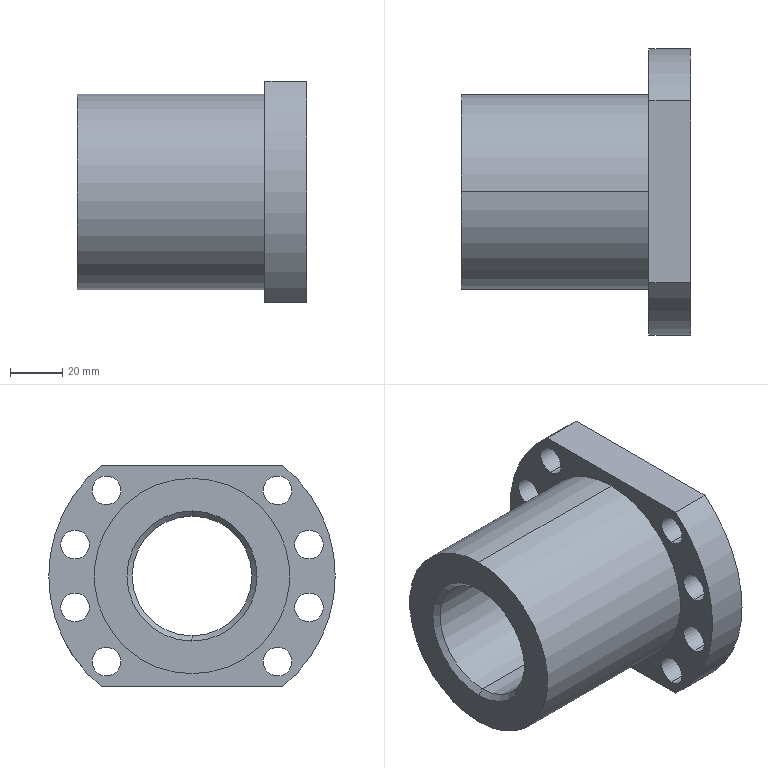Part | SolidWorks | features ICE 9, RefAxis 4, 3DProfileFeature 1, LockFeature 1, RevCut 1, Revolution 1 | 1 solid | 38 faces | box 88 x 110 x 85 mm | volume 291032 mm3 | cylinder 26 | cone 6 | plane 6 | commonest cylinder face diameters 11 x16 6 x2 6.647 x2 46 x2 75 x2 110 x2
STEP:
#1=CARTESIAN_POINT('',(80.,48.707,-24.284));
#2=VERTEX_POINT('',#1);
#3=CARTESIAN_POINT('',(80.,45.384,-30.04));
#4=VERTEX_POINT('',#3);
#5=CARTESIAN_POINT('',(80.,47.046,-27.162));
#6=DIRECTION('',(0.,-0.866,0.5));
#7=DIRECTION('',(0.,-0.5,-0.866));
#8=AXIS2_PLACEMENT_3D('',#5,#6,#7);
#9=CIRCLE('',#8,3.323);
#10=EDGE_CURVE('',#2,#4,#9,.T.);
#11=ORIENTED_EDGE('',*,*,#10,.F.);
#12=CARTESIAN_POINT('',(80.,35.437,-16.622));
#13=VERTEX_POINT('',#12);
#14=CARTESIAN_POINT('',(80.,49.293,-24.622));
#15=DIRECTION('',(0.,-0.866,0.5));
#16=VECTOR('',#15,1000.);
#17=LINE('',#14,#16);
#18=EDGE_CURVE('',#2,#13,#17,.T.);
#19=ORIENTED_EDGE('',*,*,#18,.T.);
#20=CARTESIAN_POINT('',(80.,32.113,-22.378));
#21=VERTEX_POINT('',#20);
#22=CARTESIAN_POINT('',(80.,33.775,-19.5));
#23=DIRECTION('',(0.,-0.866,0.5));
#24=DIRECTION('',(0.,-0.5,-0.866));
#25=AXIS2_PLACEMENT_3D('',#22,#23,#24);
#26=CIRCLE('',#25,3.323);
#27=EDGE_CURVE('',#13,#21,#26,.T.);
#28=ORIENTED_EDGE('',*,*,#27,.T.);
#29=CARTESIAN_POINT('',(80.,45.97,-30.378));
#30=DIRECTION('',(0.,-0.866,0.5));
#31=VECTOR('',#30,1000.);
#32=LINE('',#29,#31);
#33=EDGE_CURVE('',#4,#21,#32,.T.);
#34=ORIENTED_EDGE('',*,*,#33,.F.);
#35=EDGE_LOOP('',(#11,#19,#28,#34));
#36=FACE_OUTER_BOUND('',#35,.T.);
#37=CARTESIAN_POINT('',(80.,47.631,-27.5));
#38=DIRECTION('',(0.,-0.866,0.5));
#39=DIRECTION('',(0.,-0.5,-0.866));
#40=AXIS2_PLACEMENT_3D('',#37,#38,#39);
#41=CYLINDRICAL_SURFACE('',#40,3.323);
#42=ADVANCED_FACE('',(#36),#41,.F.);
#43=CARTESIAN_POINT('',(80.,35.275,-16.902));
#44=VERTEX_POINT('',#43);
#45=CARTESIAN_POINT('',(80.,32.275,-22.098));
#46=VERTEX_POINT('',#45);
#47=CARTESIAN_POINT('',(80.,33.775,-19.5));
#48=DIRECTION('',(0.,-0.866,0.5));
#49=DIRECTION('',(0.,-0.5,-0.866));
#50=AXIS2_PLACEMENT_3D('',#47,#48,#49);
#51=CIRCLE('',#50,3.);
#52=EDGE_CURVE('',#44,#46,#51,.T.);
#53=ORIENTED_EDGE('',*,*,#52,.F.);
#54=CARTESIAN_POINT('',(80.,21.248,-8.804));
#55=VERTEX_POINT('',#54);
#56=CARTESIAN_POINT('',(80.,49.131,-24.902));
#57=DIRECTION('',(0.,-0.866,0.5));
#58=VECTOR('',#57,1000.);
#59=LINE('',#56,#58);
#60=EDGE_CURVE('',#44,#55,#59,.T.);
#61=ORIENTED_EDGE('',*,*,#60,.T.);
#62=CARTESIAN_POINT('',(80.,18.248,-14.));
#63=VERTEX_POINT('',#62);
#64=CARTESIAN_POINT('',(80.,21.248,-8.804));
#65=CARTESIAN_POINT('',(79.804,21.248,-8.804));
#66=CARTESIAN_POINT('',(79.609,21.241,-8.821));
#67=CARTESIAN_POINT('',(79.222,21.211,-8.893));
#68=CARTESIAN_POINT('',(79.033,21.189,-8.947));
#69=CARTESIAN_POINT('',(78.672,21.13,-9.085));
#70=CARTESIAN_POINT('',(78.497,21.093,-9.171));
#71=CARTESIAN_POINT('',(78.169,21.004,-9.373));
#72=CARTESIAN_POINT('',(78.018,20.953,-9.487));
#73=CARTESIAN_POINT('',(77.742,20.837,-9.739));
#74=CARTESIAN_POINT('',(77.615,20.771,-9.879));
#75=CARTESIAN_POINT('',(77.397,20.629,-10.172));
#76=CARTESIAN_POINT('',(77.305,20.552,-10.327));
#77=CARTESIAN_POINT('',(77.154,20.386,-10.65));
#78=CARTESIAN_POINT('',(77.096,20.297,-10.819));
#79=CARTESIAN_POINT('',(77.02,20.114,-11.156));
#80=CARTESIAN_POINT('',(77.,20.019,-11.326));
#81=CARTESIAN_POINT('',(77.,19.82,-11.67));
#82=CARTESIAN_POINT('',(77.019,19.721,-11.838));
#83=CARTESIAN_POINT('',(77.095,19.52,-12.165));
#84=CARTESIAN_POINT('',(77.153,19.419,-12.327));
#85=CARTESIAN_POINT('',(77.303,19.221,-12.632));
#86=CARTESIAN_POINT('',(77.395,19.126,-12.776));
#87=CARTESIAN_POINT('',(77.613,18.942,-13.047));
#88=CARTESIAN_POINT('',(77.739,18.854,-13.174));
#89=CARTESIAN_POINT('',(78.015,18.694,-13.4));
#90=CARTESIAN_POINT('',(78.166,18.62,-13.501));
#91=CARTESIAN_POINT('',(78.494,18.49,-13.68));
#92=CARTESIAN_POINT('',(78.668,18.434,-13.755));
#93=CARTESIAN_POINT('',(79.029,18.343,-13.876));
#94=CARTESIAN_POINT('',(79.218,18.308,-13.922));
#95=CARTESIAN_POINT('',(79.605,18.26,-13.984));
#96=CARTESIAN_POINT('',(79.802,18.248,-14.));
#97=CARTESIAN_POINT('',(80.,18.248,-14.));
#98=B_SPLINE_CURVE_WITH_KNOTS('',3,(#64,#65,#66,#67,#68,#69,#70,#71,#72,#73,#74,#75,#76,#77,#78,#79,#80,#81,#82,#83,#84,#85,#86,#87,#88,#89,#90,#91,#92,#93,#94,#95,#96,#97),.UNSPECIFIED.,.F.,.F.,(4,2,2,2,2,2,2,2,2,2,2,2,2,2,2,2,4),(0.009389,0.009976,0.01056,0.01115,0.01174,0.01232,0.01291,0.0135,0.01408,0.01467,0.01526,0.01584,0.01643,0.01702,0.0176,0.01819,0.01878),.UNSPECIFIED.);
#99=EDGE_CURVE('',#55,#63,#98,.T.);
#100=ORIENTED_EDGE('',*,*,#99,.T.);
#101=CARTESIAN_POINT('',(80.,46.131,-30.098));
#102=DIRECTION('',(0.,-0.866,0.5));
#103=VECTOR('',#102,1000.);
#104=LINE('',#101,#103);
#105=EDGE_CURVE('',#46,#63,#104,.T.);
#106=ORIENTED_EDGE('',*,*,#105,.F.);
#107=EDGE_LOOP('',(#53,#61,#100,#106));
#108=FACE_OUTER_BOUND('',#107,.T.);
#109=CARTESIAN_POINT('',(80.,47.631,-27.5));
#110=DIRECTION('',(0.,-0.866,0.5));
#111=DIRECTION('',(0.,-0.5,-0.866));
#112=AXIS2_PLACEMENT_3D('',#109,#110,#111);
#113=CYLINDRICAL_SURFACE('',#112,3.);
#114=ADVANCED_FACE('',(#108),#113,.F.);
#115=ORIENTED_EDGE('',*,*,#10,.T.);
#116=CARTESIAN_POINT('',(80.,45.582,-30.778));
#117=VERTEX_POINT('',#116);
#118=CARTESIAN_POINT('',(80.,45.631,-30.964));
#119=DIRECTION('',(0.,0.2588,-0.9659));
#120=VECTOR('',#119,1000.);
#121=LINE('',#118,#120);
#122=EDGE_CURVE('',#4,#117,#121,.T.);
#123=ORIENTED_EDGE('',*,*,#122,.T.);
#124=CARTESIAN_POINT('',(80.,49.446,-24.086));
#125=VERTEX_POINT('',#124);
#126=CARTESIAN_POINT('',(80.,45.582,-30.778));
#127=CARTESIAN_POINT('',(79.744,45.582,-30.778));
#128=CARTESIAN_POINT('',(79.488,45.595,-30.759));
#129=CARTESIAN_POINT('',(78.981,45.648,-30.679));
#130=CARTESIAN_POINT('',(78.731,45.689,-30.619));
#131=CARTESIAN_POINT('',(78.017,45.845,-30.385));
#132=CARTESIAN_POINT('',(77.571,46.001,-30.151));
#133=CARTESIAN_POINT('',(77.01,46.29,-29.703));
#134=CARTESIAN_POINT('',(76.84,46.396,-29.537));
#135=CARTESIAN_POINT('',(76.544,46.621,-29.181));
#136=CARTESIAN_POINT('',(76.417,46.74,-28.99));
#137=CARTESIAN_POINT('',(76.21,46.989,-28.585));
#138=CARTESIAN_POINT('',(76.132,47.115,-28.377));
#139=CARTESIAN_POINT('',(76.027,47.372,-27.946));
#140=CARTESIAN_POINT('',(76.,47.504,-27.721));
#141=CARTESIAN_POINT('',(76.,47.761,-27.276));
#142=CARTESIAN_POINT('',(76.027,47.887,-27.054));
#143=CARTESIAN_POINT('',(76.133,48.133,-26.613));
#144=CARTESIAN_POINT('',(76.212,48.253,-26.396));
#145=CARTESIAN_POINT('',(76.417,48.476,-25.983));
#146=CARTESIAN_POINT('',(76.545,48.583,-25.783));
#147=CARTESIAN_POINT('',(76.842,48.779,-25.409));
#148=CARTESIAN_POINT('',(77.01,48.869,-25.237));
#149=CARTESIAN_POINT('',(77.383,49.03,-24.922));
#150=CARTESIAN_POINT('',(77.589,49.103,-24.778));
#151=CARTESIAN_POINT('',(78.022,49.226,-24.532));
#152=CARTESIAN_POINT('',(78.251,49.278,-24.428));
#153=CARTESIAN_POINT('',(78.731,49.362,-24.258));
#154=CARTESIAN_POINT('',(78.981,49.393,-24.193));
#155=CARTESIAN_POINT('',(79.484,49.435,-24.108));
#156=CARTESIAN_POINT('',(79.741,49.446,-24.086));
#157=CARTESIAN_POINT('',(80.,49.446,-24.086));
#158=B_SPLINE_CURVE_WITH_KNOTS('',3,(#126,#127,#128,#129,#130,#131,#132,#133,#134,#135,#136,#137,#138,#139,#140,#141,#142,#143,#144,#145,#146,#147,#148,#149,#150,#151,#152,#153,#154,#155,#156,#157),.UNSPECIFIED.,.F.,.F.,(4,2,2,2,2,2,2,2,2,2,2,2,2,2,2,4),(0.0213,0.02207,0.02284,0.02438,0.02515,0.02592,0.02669,0.02746,0.02823,0.029,0.02977,0.03054,0.03131,0.03208,0.03285,0.03363),.UNSPECIFIED.);
#159=EDGE_CURVE('',#117,#125,#158,.T.);
#160=ORIENTED_EDGE('',*,*,#159,.T.);
#161=CARTESIAN_POINT('',(80.,49.631,-24.036));
#162=DIRECTION('',(0.,0.9659,0.2588));
#163=VECTOR('',#162,1000.);
#164=LINE('',#161,#163);
#165=EDGE_CURVE('',#2,#125,#164,.T.);
#166=ORIENTED_EDGE('',*,*,#165,.F.);
#167=EDGE_LOOP('',(#115,#123,#160,#166));
#168=FACE_OUTER_BOUND('',#167,.T.);
#169=CARTESIAN_POINT('',(80.,47.631,-27.5));
#170=DIRECTION('',(0.,0.866,-0.5));
#171=DIRECTION('',(0.,0.5,0.866));
#172=AXIS2_PLACEMENT_3D('',#169,#170,#171);
#173=CONICAL_SURFACE('',#172,4.,0.7854);
#174=ADVANCED_FACE('',(#168),#173,.F.);
#175=CARTESIAN_POINT('',(72.,-32.88,38.38));
#176=VERTEX_POINT('',#175);
#177=CARTESIAN_POINT('',(72.,-32.88,27.38));
#178=VERTEX_POINT('',#177);
#179=CARTESIAN_POINT('',(72.,-32.88,32.88));
#180=DIRECTION('',(1.,0.,0.));
#181=DIRECTION('',(0.,0.,-1.));
#182=AXIS2_PLACEMENT_3D('',#179,#180,#181);
#183=CIRCLE('',#182,5.5);
#184=EDGE_CURVE('',#176,#178,#183,.T.);
#185=ORIENTED_EDGE('',*,*,#184,.F.);
#186=CARTESIAN_POINT('',(88.,-32.88,38.38));
#187=VERTEX_POINT('',#186);
#188=CARTESIAN_POINT('',(-88.,-32.88,38.38));
#189=DIRECTION('',(1.,0.,0.));
#190=VECTOR('',#189,1000.);
#191=LINE('',#188,#190);
#192=EDGE_CURVE('',#176,#187,#191,.T.);
#193=ORIENTED_EDGE('',*,*,#192,.T.);
#194=CARTESIAN_POINT('',(88.,-32.88,27.38));
#195=VERTEX_POINT('',#194);
#196=CARTESIAN_POINT('',(88.,-32.88,32.88));
#197=DIRECTION('',(1.,0.,0.));
#198=DIRECTION('',(0.,0.,-1.));
#199=AXIS2_PLACEMENT_3D('',#196,#197,#198);
#200=CIRCLE('',#199,5.5);
#201=EDGE_CURVE('',#187,#195,#200,.T.);
#202=ORIENTED_EDGE('',*,*,#201,.T.);
#203=CARTESIAN_POINT('',(-88.,-32.88,27.38));
#204=DIRECTION('',(1.,0.,0.));
#205=VECTOR('',#204,1000.);
#206=LINE('',#203,#205);
#207=EDGE_CURVE('',#178,#195,#206,.T.);
#208=ORIENTED_EDGE('',*,*,#207,.F.);
#209=EDGE_LOOP('',(#185,#193,#202,#208));
#210=FACE_OUTER_BOUND('',#209,.T.);
#211=CARTESIAN_POINT('',(-88.,-32.88,32.88));
#212=DIRECTION('',(1.,0.,0.));
#213=DIRECTION('',(0.,0.,-1.));
#214=AXIS2_PLACEMENT_3D('',#211,#212,#213);
#215=CYLINDRICAL_SURFACE('',#214,5.5);
#216=ADVANCED_FACE('',(#210),#215,.F.);
#217=CARTESIAN_POINT('',(72.,-44.916,17.535));
#218=VERTEX_POINT('',#217);
#219=CARTESIAN_POINT('',(72.,-44.916,6.535));
#220=VERTEX_POINT('',#219);
#221=CARTESIAN_POINT('',(72.,-44.916,12.035));
#222=DIRECTION('',(1.,0.,0.));
#223=DIRECTION('',(0.,0.,-1.));
#224=AXIS2_PLACEMENT_3D('',#221,#222,#223);
#225=CIRCLE('',#224,5.5);
#226=EDGE_CURVE('',#218,#220,#225,.T.);
#227=ORIENTED_EDGE('',*,*,#226,.F.);
#228=CARTESIAN_POINT('',(88.,-44.916,17.535));
#229=VERTEX_POINT('',#228);
#230=CARTESIAN_POINT('',(-88.,-44.916,17.535));
#231=DIRECTION('',(1.,0.,0.));
#232=VECTOR('',#231,1000.);
#233=LINE('',#230,#232);
#234=EDGE_CURVE('',#218,#229,#233,.T.);
#235=ORIENTED_EDGE('',*,*,#234,.T.);
#236=CARTESIAN_POINT('',(88.,-44.916,6.535));
#237=VERTEX_POINT('',#236);
#238=CARTESIAN_POINT('',(88.,-44.916,12.035));
#239=DIRECTION('',(1.,0.,0.));
#240=DIRECTION('',(0.,0.,-1.));
#241=AXIS2_PLACEMENT_3D('',#238,#239,#240);
#242=CIRCLE('',#241,5.5);
#243=EDGE_CURVE('',#229,#237,#242,.T.);
#244=ORIENTED_EDGE('',*,*,#243,.T.);
#245=CARTESIAN_POINT('',(-88.,-44.916,6.535));
#246=DIRECTION('',(1.,0.,0.));
#247=VECTOR('',#246,1000.);
#248=LINE('',#245,#247);
#249=EDGE_CURVE('',#220,#237,#248,.T.);
#250=ORIENTED_EDGE('',*,*,#249,.F.);
#251=EDGE_LOOP('',(#227,#235,#244,#250));
#252=FACE_OUTER_BOUND('',#251,.T.);
#253=CARTESIAN_POINT('',(-88.,-44.916,12.035));
#254=DIRECTION('',(1.,0.,0.));
#255=DIRECTION('',(0.,0.,-1.));
#256=AXIS2_PLACEMENT_3D('',#253,#254,#255);
#257=CYLINDRICAL_SURFACE('',#256,5.5);
#258=ADVANCED_FACE('',(#252),#257,.F.);
#259=CARTESIAN_POINT('',(72.,-44.916,-6.535));
#260=VERTEX_POINT('',#259);
#261=CARTESIAN_POINT('',(72.,-44.916,-17.535));
#262=VERTEX_POINT('',#261);
#263=CARTESIAN_POINT('',(72.,-44.916,-12.035));
#264=DIRECTION('',(1.,0.,0.));
#265=DIRECTION('',(0.,0.,-1.));
#266=AXIS2_PLACEMENT_3D('',#263,#264,#265);
#267=CIRCLE('',#266,5.5);
#268=EDGE_CURVE('',#260,#262,#267,.T.);
#269=ORIENTED_EDGE('',*,*,#268,.F.);
#270=CARTESIAN_POINT('',(88.,-44.916,-6.535));
#271=VERTEX_POINT('',#270);
#272=CARTESIAN_POINT('',(-88.,-44.916,-6.535));
#273=DIRECTION('',(1.,0.,0.));
#274=VECTOR('',#273,1000.);
#275=LINE('',#272,#274);
#276=EDGE_CURVE('',#260,#271,#275,.T.);
#277=ORIENTED_EDGE('',*,*,#276,.T.);
#278=CARTESIAN_POINT('',(88.,-44.916,-17.535));
#279=VERTEX_POINT('',#278);
#280=CARTESIAN_POINT('',(88.,-44.916,-12.035));
#281=DIRECTION('',(1.,0.,0.));
#282=DIRECTION('',(0.,0.,-1.));
#283=AXIS2_PLACEMENT_3D('',#280,#281,#282);
#284=CIRCLE('',#283,5.5);
#285=EDGE_CURVE('',#271,#279,#284,.T.);
#286=ORIENTED_EDGE('',*,*,#285,.T.);
#287=CARTESIAN_POINT('',(-88.,-44.916,-17.535));
#288=DIRECTION('',(1.,0.,0.));
#289=VECTOR('',#288,1000.);
#290=LINE('',#287,#289);
#291=EDGE_CURVE('',#262,#279,#290,.T.);
#292=ORIENTED_EDGE('',*,*,#291,.F.);
#293=EDGE_LOOP('',(#269,#277,#286,#292));
#294=FACE_OUTER_BOUND('',#293,.T.);
#295=CARTESIAN_POINT('',(-88.,-44.916,-12.035));
#296=DIRECTION('',(1.,0.,0.));
#297=DIRECTION('',(0.,0.,-1.));
#298=AXIS2_PLACEMENT_3D('',#295,#296,#297);
#299=CYLINDRICAL_SURFACE('',#298,5.5);
#300=ADVANCED_FACE('',(#294),#299,.F.);
#301=CARTESIAN_POINT('',(72.,-32.88,-27.38));
#302=VERTEX_POINT('',#301);
#303=CARTESIAN_POINT('',(72.,-32.88,-38.38));
#304=VERTEX_POINT('',#303);
#305=CARTESIAN_POINT('',(72.,-32.88,-32.88));
#306=DIRECTION('',(1.,0.,0.));
#307=DIRECTION('',(0.,0.,-1.));
#308=AXIS2_PLACEMENT_3D('',#305,#306,#307);
#309=CIRCLE('',#308,5.5);
#310=EDGE_CURVE('',#302,#304,#309,.T.);
#311=ORIENTED_EDGE('',*,*,#310,.F.);
#312=CARTESIAN_POINT('',(88.,-32.88,-27.38));
#313=VERTEX_POINT('',#312);
#314=CARTESIAN_POINT('',(-88.,-32.88,-27.38));
#315=DIRECTION('',(1.,0.,0.));
#316=VECTOR('',#315,1000.);
#317=LINE('',#314,#316);
#318=EDGE_CURVE('',#302,#313,#317,.T.);
#319=ORIENTED_EDGE('',*,*,#318,.T.);
#320=CARTESIAN_POINT('',(88.,-32.88,-38.38));
#321=VERTEX_POINT('',#320);
#322=CARTESIAN_POINT('',(88.,-32.88,-32.88));
#323=DIRECTION('',(1.,0.,0.));
#324=DIRECTION('',(0.,0.,-1.));
#325=AXIS2_PLACEMENT_3D('',#322,#323,#324);
#326=CIRCLE('',#325,5.5);
#327=EDGE_CURVE('',#313,#321,#326,.T.);
#328=ORIENTED_EDGE('',*,*,#327,.T.);
#329=CARTESIAN_POINT('',(-88.,-32.88,-38.38));
#330=DIRECTION('',(1.,0.,0.));
#331=VECTOR('',#330,1000.);
#332=LINE('',#329,#331);
#333=EDGE_CURVE('',#304,#321,#332,.T.);
#334=ORIENTED_EDGE('',*,*,#333,.F.);
#335=EDGE_LOOP('',(#311,#319,#328,#334));
#336=FACE_OUTER_BOUND('',#335,.T.);
#337=CARTESIAN_POINT('',(-88.,-32.88,-32.88));
#338=DIRECTION('',(1.,0.,0.));
#339=DIRECTION('',(0.,0.,-1.));
#340=AXIS2_PLACEMENT_3D('',#337,#338,#339);
#341=CYLINDRICAL_SURFACE('',#340,5.5);
#342=ADVANCED_FACE('',(#336),#341,.F.);
#343=CARTESIAN_POINT('',(72.,32.88,-27.38));
#344=VERTEX_POINT('',#343);
#345=CARTESIAN_POINT('',(72.,32.88,-38.38));
#346=VERTEX_POINT('',#345);
#347=CARTESIAN_POINT('',(72.,32.88,-32.88));
#348=DIRECTION('',(1.,0.,0.));
#349=DIRECTION('',(0.,0.,-1.));
#350=AXIS2_PLACEMENT_3D('',#347,#348,#349);
#351=CIRCLE('',#350,5.5);
#352=EDGE_CURVE('',#344,#346,#351,.T.);
#353=ORIENTED_EDGE('',*,*,#352,.F.);
#354=CARTESIAN_POINT('',(88.,32.88,-27.38));
#355=VERTEX_POINT('',#354);
#356=CARTESIAN_POINT('',(-88.,32.88,-27.38));
#357=DIRECTION('',(1.,0.,0.));
#358=VECTOR('',#357,1000.);
#359=LINE('',#356,#358);
#360=EDGE_CURVE('',#344,#355,#359,.T.);
#361=ORIENTED_EDGE('',*,*,#360,.T.);
#362=CARTESIAN_POINT('',(88.,32.88,-38.38));
#363=VERTEX_POINT('',#362);
#364=CARTESIAN_POINT('',(88.,32.88,-32.88));
#365=DIRECTION('',(1.,0.,0.));
#366=DIRECTION('',(0.,0.,-1.));
#367=AXIS2_PLACEMENT_3D('',#364,#365,#366);
#368=CIRCLE('',#367,5.5);
#369=EDGE_CURVE('',#355,#363,#368,.T.);
#370=ORIENTED_EDGE('',*,*,#369,.T.);
#371=CARTESIAN_POINT('',(-88.,32.88,-38.38));
#372=DIRECTION('',(1.,0.,0.));
#373=VECTOR('',#372,1000.);
#374=LINE('',#371,#373);
#375=EDGE_CURVE('',#346,#363,#374,.T.);
#376=ORIENTED_EDGE('',*,*,#375,.F.);
#377=EDGE_LOOP('',(#353,#361,#370,#376));
#378=FACE_OUTER_BOUND('',#377,.T.);
#379=CARTESIAN_POINT('',(-88.,32.88,-32.88));
#380=DIRECTION('',(1.,0.,0.));
#381=DIRECTION('',(0.,0.,-1.));
#382=AXIS2_PLACEMENT_3D('',#379,#380,#381);
#383=CYLINDRICAL_SURFACE('',#382,5.5);
#384=ADVANCED_FACE('',(#378),#383,.F.);
#385=CARTESIAN_POINT('',(72.,44.916,-6.535));
#386=VERTEX_POINT('',#385);
#387=CARTESIAN_POINT('',(72.,44.916,-17.535));
#388=VERTEX_POINT('',#387);
#389=CARTESIAN_POINT('',(72.,44.916,-12.035));
#390=DIRECTION('',(1.,0.,0.));
#391=DIRECTION('',(0.,0.,-1.));
#392=AXIS2_PLACEMENT_3D('',#389,#390,#391);
#393=CIRCLE('',#392,5.5);
#394=EDGE_CURVE('',#386,#388,#393,.T.);
#395=ORIENTED_EDGE('',*,*,#394,.F.);
#396=CARTESIAN_POINT('',(88.,44.916,-6.535));
#397=VERTEX_POINT('',#396);
#398=CARTESIAN_POINT('',(-88.,44.916,-6.535));
#399=DIRECTION('',(1.,0.,0.));
#400=VECTOR('',#399,1000.);
#401=LINE('',#398,#400);
#402=EDGE_CURVE('',#386,#397,#401,.T.);
#403=ORIENTED_EDGE('',*,*,#402,.T.);
#404=CARTESIAN_POINT('',(88.,44.916,-17.535));
#405=VERTEX_POINT('',#404);
#406=CARTESIAN_POINT('',(88.,44.916,-12.035));
#407=DIRECTION('',(1.,0.,0.));
#408=DIRECTION('',(0.,0.,-1.));
#409=AXIS2_PLACEMENT_3D('',#406,#407,#408);
#410=CIRCLE('',#409,5.5);
#411=EDGE_CURVE('',#397,#405,#410,.T.);
#412=ORIENTED_EDGE('',*,*,#411,.T.);
#413=CARTESIAN_POINT('',(-88.,44.916,-17.535));
#414=DIRECTION('',(1.,0.,0.));
#415=VECTOR('',#414,1000.);
#416=LINE('',#413,#415);
#417=EDGE_CURVE('',#388,#405,#416,.T.);
#418=ORIENTED_EDGE('',*,*,#417,.F.);
#419=EDGE_LOOP('',(#395,#403,#412,#418));
#420=FACE_OUTER_BOUND('',#419,.T.);
#421=CARTESIAN_POINT('',(-88.,44.916,-12.035));
#422=DIRECTION('',(1.,0.,0.));
#423=DIRECTION('',(0.,0.,-1.));
#424=AXIS2_PLACEMENT_3D('',#421,#422,#423);
#425=CYLINDRICAL_SURFACE('',#424,5.5);
#426=ADVANCED_FACE('',(#420),#425,.F.);
#427=CARTESIAN_POINT('',(72.,44.916,17.535));
#428=VERTEX_POINT('',#427);
#429=CARTESIAN_POINT('',(72.,44.916,6.535));
#430=VERTEX_POINT('',#429);
#431=CARTESIAN_POINT('',(72.,44.916,12.035));
#432=DIRECTION('',(1.,0.,0.));
#433=DIRECTION('',(0.,0.,-1.));
#434=AXIS2_PLACEMENT_3D('',#431,#432,#433);
#435=CIRCLE('',#434,5.5);
#436=EDGE_CURVE('',#428,#430,#435,.T.);
#437=ORIENTED_EDGE('',*,*,#436,.F.);
#438=CARTESIAN_POINT('',(88.,44.916,17.535));
#439=VERTEX_POINT('',#438);
#440=CARTESIAN_POINT('',(-88.,44.916,17.535));
#441=DIRECTION('',(1.,0.,0.));
#442=VECTOR('',#441,1000.);
#443=LINE('',#440,#442);
#444=EDGE_CURVE('',#428,#439,#443,.T.);
#445=ORIENTED_EDGE('',*,*,#444,.T.);
#446=CARTESIAN_POINT('',(88.,44.916,6.535));
#447=VERTEX_POINT('',#446);
#448=CARTESIAN_POINT('',(88.,44.916,12.035));
#449=DIRECTION('',(1.,0.,0.));
#450=DIRECTION('',(0.,0.,-1.));
#451=AXIS2_PLACEMENT_3D('',#448,#449,#450);
#452=CIRCLE('',#451,5.5);
#453=EDGE_CURVE('',#439,#447,#452,.T.);
#454=ORIENTED_EDGE('',*,*,#453,.T.);
#455=CARTESIAN_POINT('',(-88.,44.916,6.535));
#456=DIRECTION('',(1.,0.,0.));
#457=VECTOR('',#456,1000.);
#458=LINE('',#455,#457);
#459=EDGE_CURVE('',#430,#447,#458,.T.);
#460=ORIENTED_EDGE('',*,*,#459,.F.);
#461=EDGE_LOOP('',(#437,#445,#454,#460));
#462=FACE_OUTER_BOUND('',#461,.T.);
#463=CARTESIAN_POINT('',(-88.,44.916,12.035));
#464=DIRECTION('',(1.,0.,0.));
#465=DIRECTION('',(0.,0.,-1.));
#466=AXIS2_PLACEMENT_3D('',#463,#464,#465);
#467=CYLINDRICAL_SURFACE('',#466,5.5);
#468=ADVANCED_FACE('',(#462),#467,.F.);
#469=CARTESIAN_POINT('',(72.,32.88,38.38));
#470=VERTEX_POINT('',#469);
#471=CARTESIAN_POINT('',(72.,32.88,27.38));
#472=VERTEX_POINT('',#471);
#473=CARTESIAN_POINT('',(72.,32.88,32.88));
#474=DIRECTION('',(1.,0.,0.));
#475=DIRECTION('',(0.,0.,-1.));
#476=AXIS2_PLACEMENT_3D('',#473,#474,#475);
#477=CIRCLE('',#476,5.5);
#478=EDGE_CURVE('',#470,#472,#477,.T.);
#479=ORIENTED_EDGE('',*,*,#478,.F.);
#480=CARTESIAN_POINT('',(88.,32.88,38.38));
#481=VERTEX_POINT('',#480);
#482=CARTESIAN_POINT('',(-88.,32.88,38.38));
#483=DIRECTION('',(1.,0.,0.));
#484=VECTOR('',#483,1000.);
#485=LINE('',#482,#484);
#486=EDGE_CURVE('',#470,#481,#485,.T.);
#487=ORIENTED_EDGE('',*,*,#486,.T.);
#488=CARTESIAN_POINT('',(88.,32.88,27.38));
#489=VERTEX_POINT('',#488);
#490=CARTESIAN_POINT('',(88.,32.88,32.88));
#491=DIRECTION('',(1.,0.,0.));
#492=DIRECTION('',(0.,0.,-1.));
#493=AXIS2_PLACEMENT_3D('',#490,#491,#492);
#494=CIRCLE('',#493,5.5);
#495=EDGE_CURVE('',#481,#489,#494,.T.);
#496=ORIENTED_EDGE('',*,*,#495,.T.);
#497=CARTESIAN_POINT('',(-88.,32.88,27.38));
#498=DIRECTION('',(1.,0.,0.));
#499=VECTOR('',#498,1000.);
#500=LINE('',#497,#499);
#501=EDGE_CURVE('',#472,#489,#500,.T.);
#502=ORIENTED_EDGE('',*,*,#501,.F.);
#503=EDGE_LOOP('',(#479,#487,#496,#502));
#504=FACE_OUTER_BOUND('',#503,.T.);
#505=CARTESIAN_POINT('',(-88.,32.88,32.88));
#506=DIRECTION('',(1.,0.,0.));
#507=DIRECTION('',(0.,0.,-1.));
#508=AXIS2_PLACEMENT_3D('',#505,#506,#507);
#509=CYLINDRICAL_SURFACE('',#508,5.5);
#510=ADVANCED_FACE('',(#504),#509,.F.);
#511=CARTESIAN_POINT('',(86.,0.,-23.));
#512=VERTEX_POINT('',#511);
#513=CARTESIAN_POINT('',(86.,0.,23.));
#514=VERTEX_POINT('',#513);
#515=CARTESIAN_POINT('',(86.,0.,0.));
#516=DIRECTION('',(-1.,0.,0.));
#517=DIRECTION('',(0.,0.,1.));
#518=AXIS2_PLACEMENT_3D('',#515,#516,#517);
#519=CIRCLE('',#518,23.);
#520=EDGE_CURVE('',#512,#514,#519,.T.);
#521=ORIENTED_EDGE('',*,*,#520,.T.);
#522=CARTESIAN_POINT('',(88.,0.,25.));
#523=VERTEX_POINT('',#522);
#524=CARTESIAN_POINT('',(86.,0.,23.));
#525=DIRECTION('',(0.7071,0.,0.7071));
#526=VECTOR('',#525,1000.);
#527=LINE('',#524,#526);
#528=EDGE_CURVE('',#514,#523,#527,.T.);
#529=ORIENTED_EDGE('',*,*,#528,.T.);
#530=CARTESIAN_POINT('',(88.,0.,-25.));
#531=VERTEX_POINT('',#530);
#532=CARTESIAN_POINT('',(88.,0.,0.));
#533=DIRECTION('',(-1.,0.,0.));
#534=DIRECTION('',(0.,0.,1.));
#535=AXIS2_PLACEMENT_3D('',#532,#533,#534);
#536=CIRCLE('',#535,25.);
#537=EDGE_CURVE('',#531,#523,#536,.T.);
#538=ORIENTED_EDGE('',*,*,#537,.F.);
#539=CARTESIAN_POINT('',(86.,0.,-23.));
#540=DIRECTION('',(0.7071,0.,-0.7071));
#541=VECTOR('',#540,1000.);
#542=LINE('',#539,#541);
#543=EDGE_CURVE('',#512,#531,#542,.T.);
#544=ORIENTED_EDGE('',*,*,#543,.F.);
#545=EDGE_LOOP('',(#521,#529,#538,#544));
#546=FACE_OUTER_BOUND('',#545,.T.);
#547=CARTESIAN_POINT('',(86.,0.,0.));
#548=DIRECTION('',(1.,0.,0.));
#549=DIRECTION('',(0.,0.,-1.));
#550=AXIS2_PLACEMENT_3D('',#547,#548,#549);
#551=CONICAL_SURFACE('',#550,23.,0.7854);
#552=ADVANCED_FACE('',(#546),#551,.F.);
#553=CARTESIAN_POINT('',(2.,0.,-23.));
#554=VERTEX_POINT('',#553);
#555=CARTESIAN_POINT('',(2.,0.,23.));
#556=VERTEX_POINT('',#555);
#557=CARTESIAN_POINT('',(2.,0.,0.));
#558=DIRECTION('',(-1.,0.,0.));
#559=DIRECTION('',(0.,0.,1.));
#560=AXIS2_PLACEMENT_3D('',#557,#558,#559);
#561=CIRCLE('',#560,23.);
#562=EDGE_CURVE('',#554,#556,#561,.T.);
#563=ORIENTED_EDGE('',*,*,#562,.F.);
#564=CARTESIAN_POINT('',(0.,0.,-25.));
#565=VERTEX_POINT('',#564);
#566=CARTESIAN_POINT('',(0.,0.,-25.));
#567=DIRECTION('',(-0.7071,0.,-0.7071));
#568=VECTOR('',#567,1000.);
#569=LINE('',#566,#568);
#570=EDGE_CURVE('',#554,#565,#569,.T.);
#571=ORIENTED_EDGE('',*,*,#570,.T.);
#572=CARTESIAN_POINT('',(0.,0.,25.));
#573=VERTEX_POINT('',#572);
#574=CARTESIAN_POINT('',(0.,0.,0.));
#575=DIRECTION('',(-1.,0.,0.));
#576=DIRECTION('',(0.,0.,1.));
#577=AXIS2_PLACEMENT_3D('',#574,#575,#576);
#578=CIRCLE('',#577,25.);
#579=EDGE_CURVE('',#565,#573,#578,.T.);
#580=ORIENTED_EDGE('',*,*,#579,.T.);
#581=CARTESIAN_POINT('',(0.,0.,25.));
#582=DIRECTION('',(-0.7071,0.,0.7071));
#583=VECTOR('',#582,1000.);
#584=LINE('',#581,#583);
#585=EDGE_CURVE('',#556,#573,#584,.T.);
#586=ORIENTED_EDGE('',*,*,#585,.F.);
#587=EDGE_LOOP('',(#563,#571,#580,#586));
#588=FACE_OUTER_BOUND('',#587,.T.);
#589=CARTESIAN_POINT('',(0.,0.,0.));
#590=DIRECTION('',(-1.,0.,0.));
#591=DIRECTION('',(0.,0.,1.));
#592=AXIS2_PLACEMENT_3D('',#589,#590,#591);
#593=CONICAL_SURFACE('',#592,25.,0.7854);
#594=ADVANCED_FACE('',(#588),#593,.F.);
#595=CARTESIAN_POINT('',(72.,0.,37.5));
#596=VERTEX_POINT('',#595);
#597=CARTESIAN_POINT('',(72.,0.,-37.5));
#598=VERTEX_POINT('',#597);
#599=CARTESIAN_POINT('',(72.,0.,0.));
#600=DIRECTION('',(-1.,0.,0.));
#601=DIRECTION('',(0.,0.,1.));
#602=AXIS2_PLACEMENT_3D('',#599,#600,#601);
#603=CIRCLE('',#602,37.5);
#604=EDGE_CURVE('',#596,#598,#603,.T.);
#605=ORIENTED_EDGE('',*,*,#604,.T.);
#606=CARTESIAN_POINT('',(0.,0.,-37.5));
#607=VERTEX_POINT('',#606);
#608=CARTESIAN_POINT('',(88.,0.,-37.5));
#609=DIRECTION('',(-1.,0.,0.));
#610=VECTOR('',#609,1000.);
#611=LINE('',#608,#610);
#612=EDGE_CURVE('',#598,#607,#611,.T.);
#613=ORIENTED_EDGE('',*,*,#612,.T.);
#614=CARTESIAN_POINT('',(0.,0.,37.5));
#615=VERTEX_POINT('',#614);
#616=CARTESIAN_POINT('',(0.,0.,0.));
#617=DIRECTION('',(-1.,0.,0.));
#618=DIRECTION('',(0.,0.,1.));
#619=AXIS2_PLACEMENT_3D('',#616,#617,#618);
#620=CIRCLE('',#619,37.5);
#621=EDGE_CURVE('',#615,#607,#620,.T.);
#622=ORIENTED_EDGE('',*,*,#621,.F.);
#623=CARTESIAN_POINT('',(88.,0.,37.5));
#624=DIRECTION('',(-1.,0.,0.));
#625=VECTOR('',#624,1000.);
#626=LINE('',#623,#625);
#627=EDGE_CURVE('',#596,#615,#626,.T.);
#628=ORIENTED_EDGE('',*,*,#627,.F.);
#629=EDGE_LOOP('',(#605,#613,#622,#628));
#630=FACE_OUTER_BOUND('',#629,.T.);
#631=CARTESIAN_POINT('',(88.,0.,0.));
#632=DIRECTION('',(-1.,0.,0.));
#633=DIRECTION('',(0.,0.,1.));
#634=AXIS2_PLACEMENT_3D('',#631,#632,#633);
#635=CYLINDRICAL_SURFACE('',#634,37.5);
#636=ADVANCED_FACE('',(#630),#635,.T.);
#637=ORIENTED_EDGE('',*,*,#520,.F.);
#638=CARTESIAN_POINT('',(88.,0.,-23.));
#639=DIRECTION('',(-1.,0.,0.));
#640=VECTOR('',#639,1000.);
#641=LINE('',#638,#640);
#642=EDGE_CURVE('',#512,#554,#641,.T.);
#643=ORIENTED_EDGE('',*,*,#642,.T.);
#644=ORIENTED_EDGE('',*,*,#562,.T.);
#645=CARTESIAN_POINT('',(88.,0.,23.));
#646=DIRECTION('',(-1.,0.,0.));
#647=VECTOR('',#646,1000.);
#648=LINE('',#645,#647);
#649=EDGE_CURVE('',#514,#556,#648,.T.);
#650=ORIENTED_EDGE('',*,*,#649,.F.);
#651=EDGE_LOOP('',(#637,#643,#644,#650));
#652=FACE_OUTER_BOUND('',#651,.T.);
#653=CARTESIAN_POINT('',(88.,0.,0.));
#654=DIRECTION('',(-1.,0.,0.));
#655=DIRECTION('',(0.,0.,1.));
#656=AXIS2_PLACEMENT_3D('',#653,#654,#655);
#657=CYLINDRICAL_SURFACE('',#656,23.);
#658=ADVANCED_FACE('',(#652),#657,.F.);
#659=CARTESIAN_POINT('',(72.,34.911,-42.5));
#660=VERTEX_POINT('',#659);
#661=CARTESIAN_POINT('',(88.,34.911,-42.5));
#662=VERTEX_POINT('',#661);
#663=CARTESIAN_POINT('',(88.,34.911,-42.5));
#664=DIRECTION('',(1.,0.,0.));
#665=VECTOR('',#664,1000.);
#666=LINE('',#663,#665);
#667=EDGE_CURVE('',#660,#662,#666,.T.);
#668=ORIENTED_EDGE('',*,*,#667,.F.);
#669=CARTESIAN_POINT('',(72.,34.911,42.5));
#670=VERTEX_POINT('',#669);
#671=CARTESIAN_POINT('',(72.,0.,0.));
#672=DIRECTION('',(-1.,0.,0.));
#673=DIRECTION('',(0.,0.,1.));
#674=AXIS2_PLACEMENT_3D('',#671,#672,#673);
#675=CIRCLE('',#674,55.);
#676=EDGE_CURVE('',#670,#660,#675,.T.);
#677=ORIENTED_EDGE('',*,*,#676,.F.);
#678=CARTESIAN_POINT('',(88.,34.911,42.5));
#679=VERTEX_POINT('',#678);
#680=CARTESIAN_POINT('',(88.,34.911,42.5));
#681=DIRECTION('',(-1.,0.,0.));
#682=VECTOR('',#681,1000.);
#683=LINE('',#680,#682);
#684=EDGE_CURVE('',#679,#670,#683,.T.);
#685=ORIENTED_EDGE('',*,*,#684,.F.);
#686=CARTESIAN_POINT('',(88.,0.,0.));
#687=DIRECTION('',(-1.,0.,0.));
#688=DIRECTION('',(0.,0.,1.));
#689=AXIS2_PLACEMENT_3D('',#686,#687,#688);
#690=CIRCLE('',#689,55.);
#691=EDGE_CURVE('',#679,#662,#690,.T.);
#692=ORIENTED_EDGE('',*,*,#691,.T.);
#693=EDGE_LOOP('',(#668,#677,#685,#692));
#694=FACE_OUTER_BOUND('',#693,.T.);
#695=CARTESIAN_POINT('',(80.,49.446,-24.086));
#696=CARTESIAN_POINT('',(80.259,49.446,-24.086));
#697=CARTESIAN_POINT('',(80.515,49.435,-24.107));
#698=CARTESIAN_POINT('',(81.018,49.393,-24.193));
#699=CARTESIAN_POINT('',(81.269,49.362,-24.258));
#700=CARTESIAN_POINT('',(81.749,49.278,-24.428));
#701=CARTESIAN_POINT('',(81.977,49.226,-24.532));
#702=CARTESIAN_POINT('',(82.41,49.103,-24.778));
#703=CARTESIAN_POINT('',(82.617,49.03,-24.921));
#704=CARTESIAN_POINT('',(82.989,48.869,-25.236));
#705=CARTESIAN_POINT('',(83.157,48.78,-25.408));
#706=CARTESIAN_POINT('',(83.454,48.584,-25.781));
#707=CARTESIAN_POINT('',(83.582,48.477,-25.982));
#708=CARTESIAN_POINT('',(83.787,48.253,-26.394));
#709=CARTESIAN_POINT('',(83.866,48.136,-26.608));
#710=CARTESIAN_POINT('',(83.973,47.888,-27.052));
#711=CARTESIAN_POINT('',(84.,47.761,-27.275));
#712=CARTESIAN_POINT('',(84.,47.505,-27.719));
#713=CARTESIAN_POINT('',(83.974,47.373,-27.943));
#714=CARTESIAN_POINT('',(83.868,47.115,-28.377));
#715=CARTESIAN_POINT('',(83.79,46.989,-28.585));
#716=CARTESIAN_POINT('',(83.584,46.741,-28.988));
#717=CARTESIAN_POINT('',(83.456,46.621,-29.181));
#718=CARTESIAN_POINT('',(83.161,46.397,-29.536));
#719=CARTESIAN_POINT('',(82.993,46.291,-29.701));
#720=CARTESIAN_POINT('',(82.616,46.097,-30.001));
#721=CARTESIAN_POINT('',(82.414,46.011,-30.133));
#722=CARTESIAN_POINT('',(81.981,45.859,-30.364));
#723=CARTESIAN_POINT('',(81.748,45.794,-30.462));
#724=CARTESIAN_POINT('',(81.269,45.689,-30.619));
#725=CARTESIAN_POINT('',(81.023,45.649,-30.679));
#726=CARTESIAN_POINT('',(80.517,45.595,-30.758));
#727=CARTESIAN_POINT('',(80.257,45.582,-30.778));
#728=CARTESIAN_POINT('',(80.,45.582,-30.778));
#729=B_SPLINE_CURVE_WITH_KNOTS('',3,(#695,#696,#697,#698,#699,#700,#701,#702,#703,#704,#705,#706,#707,#708,#709,#710,#711,#712,#713,#714,#715,#716,#717,#718,#719,#720,#721,#722,#723,#724,#725,#726,#727,#728),.UNSPECIFIED.,.F.,.F.,(4,2,2,2,2,2,2,2,2,2,2,2,2,2,2,2,4),(0.008966,0.009737,0.01051,0.01128,0.01205,0.01282,0.01359,0.01436,0.01513,0.0159,0.01667,0.01744,0.01822,0.01899,0.01976,0.02053,0.0213),.UNSPECIFIED.);
#730=EDGE_CURVE('',#125,#117,#729,.T.);
#731=ORIENTED_EDGE('',*,*,#730,.F.);
#732=ORIENTED_EDGE('',*,*,#159,.F.);
#733=EDGE_LOOP('',(#731,#732));
#734=FACE_BOUND('',#733,.T.);
#735=CARTESIAN_POINT('',(88.,0.,0.));
#736=DIRECTION('',(-1.,0.,0.));
#737=DIRECTION('',(0.,0.,1.));
#738=AXIS2_PLACEMENT_3D('',#735,#736,#737);
#739=CYLINDRICAL_SURFACE('',#738,55.);
#740=ADVANCED_FACE('',(#694,#734),#739,.T.);
#741=ORIENTED_EDGE('',*,*,#642,.F.);
#742=CARTESIAN_POINT('',(86.,0.,0.));
#743=DIRECTION('',(-1.,0.,0.));
#744=DIRECTION('',(0.,0.,1.));
#745=AXIS2_PLACEMENT_3D('',#742,#743,#744);
#746=CIRCLE('',#745,23.);
#747=EDGE_CURVE('',#514,#512,#746,.T.);
#748=ORIENTED_EDGE('',*,*,#747,.F.);
#749=ORIENTED_EDGE('',*,*,#649,.T.);
#750=CARTESIAN_POINT('',(2.,0.,0.));
#751=DIRECTION('',(-1.,0.,0.));
#752=DIRECTION('',(0.,0.,1.));
#753=AXIS2_PLACEMENT_3D('',#750,#751,#752);
#754=CIRCLE('',#753,23.);
#755=EDGE_CURVE('',#556,#554,#754,.T.);
#756=ORIENTED_EDGE('',*,*,#755,.T.);
#757=EDGE_LOOP('',(#741,#748,#749,#756));
#758=FACE_OUTER_BOUND('',#757,.T.);
#759=CARTESIAN_POINT('',(80.,18.248,-14.));
#760=CARTESIAN_POINT('',(80.198,18.248,-14.));
#761=CARTESIAN_POINT('',(80.394,18.26,-13.984));
#762=CARTESIAN_POINT('',(80.777,18.307,-13.923));
#763=CARTESIAN_POINT('',(80.968,18.342,-13.877));
#764=CARTESIAN_POINT('',(81.331,18.434,-13.755));
#765=CARTESIAN_POINT('',(81.503,18.489,-13.681));
#766=CARTESIAN_POINT('',(81.829,18.618,-13.504));
#767=CARTESIAN_POINT('',(81.984,18.693,-13.401));
#768=CARTESIAN_POINT('',(82.26,18.853,-13.174));
#769=CARTESIAN_POINT('',(82.384,18.94,-13.05));
#770=CARTESIAN_POINT('',(82.603,19.125,-12.778));
#771=CARTESIAN_POINT('',(82.696,19.221,-12.632));
#772=CARTESIAN_POINT('',(82.846,19.417,-12.329));
#773=CARTESIAN_POINT('',(82.904,19.518,-12.169));
#774=CARTESIAN_POINT('',(82.981,19.72,-11.838));
#775=CARTESIAN_POINT('',(83.,19.82,-11.671));
#776=CARTESIAN_POINT('',(83.,20.016,-11.331));
#777=CARTESIAN_POINT('',(82.981,20.113,-11.158));
#778=CARTESIAN_POINT('',(82.904,20.297,-10.819));
#779=CARTESIAN_POINT('',(82.847,20.385,-10.654));
#780=CARTESIAN_POINT('',(82.697,20.551,-10.33));
#781=CARTESIAN_POINT('',(82.603,20.629,-10.173));
#782=CARTESIAN_POINT('',(82.386,20.771,-9.879));
#783=CARTESIAN_POINT('',(82.261,20.836,-9.742));
#784=CARTESIAN_POINT('',(81.982,20.953,-9.486));
#785=CARTESIAN_POINT('',(81.83,21.004,-9.373));
#786=CARTESIAN_POINT('',(81.506,21.092,-9.173));
#787=CARTESIAN_POINT('',(81.33,21.129,-9.086));
#788=CARTESIAN_POINT('',(80.967,21.189,-8.946));
#789=CARTESIAN_POINT('',(80.78,21.211,-8.893));
#790=CARTESIAN_POINT('',(80.395,21.241,-8.822));
#791=CARTESIAN_POINT('',(80.196,21.248,-8.804));
#792=CARTESIAN_POINT('',(80.,21.248,-8.804));
#793=B_SPLINE_CURVE_WITH_KNOTS('',3,(#759,#760,#761,#762,#763,#764,#765,#766,#767,#768,#769,#770,#771,#772,#773,#774,#775,#776,#777,#778,#779,#780,#781,#782,#783,#784,#785,#786,#787,#788,#789,#790,#791,#792),.UNSPECIFIED.,.F.,.F.,(4,2,2,2,2,2,2,2,2,2,2,2,2,2,2,2,4),(0.,0.0005868,0.001174,0.001761,0.002347,0.002934,0.003521,0.004108,0.004695,0.005282,0.005868,0.006455,0.007042,0.007629,0.008216,0.008803,0.009389),.UNSPECIFIED.);
#794=EDGE_CURVE('',#63,#55,#793,.T.);
#795=ORIENTED_EDGE('',*,*,#794,.F.);
#796=ORIENTED_EDGE('',*,*,#99,.F.);
#797=EDGE_LOOP('',(#795,#796));
#798=FACE_BOUND('',#797,.T.);
#799=CARTESIAN_POINT('',(88.,0.,0.));
#800=DIRECTION('',(-1.,0.,0.));
#801=DIRECTION('',(0.,0.,1.));
#802=AXIS2_PLACEMENT_3D('',#799,#800,#801);
#803=CYLINDRICAL_SURFACE('',#802,23.);
#804=ADVANCED_FACE('',(#758,#798),#803,.F.);
#805=CARTESIAN_POINT('',(88.,-32.88,32.88));
#806=DIRECTION('',(1.,0.,0.));
#807=DIRECTION('',(0.,0.,-1.));
#808=AXIS2_PLACEMENT_3D('',#805,#806,#807);
#809=CIRCLE('',#808,5.5);
#810=EDGE_CURVE('',#195,#187,#809,.T.);
#811=ORIENTED_EDGE('',*,*,#810,.F.);
#812=ORIENTED_EDGE('',*,*,#201,.F.);
#813=EDGE_LOOP('',(#811,#812));
#814=FACE_BOUND('',#813,.T.);
#815=CARTESIAN_POINT('',(88.,-44.916,12.035));
#816=DIRECTION('',(1.,0.,0.));
#817=DIRECTION('',(0.,0.,-1.));
#818=AXIS2_PLACEMENT_3D('',#815,#816,#817);
#819=CIRCLE('',#818,5.5);
#820=EDGE_CURVE('',#237,#229,#819,.T.);
#821=ORIENTED_EDGE('',*,*,#820,.F.);
#822=ORIENTED_EDGE('',*,*,#243,.F.);
#823=EDGE_LOOP('',(#821,#822));
#824=FACE_BOUND('',#823,.T.);
#825=CARTESIAN_POINT('',(88.,-44.916,-12.035));
#826=DIRECTION('',(1.,0.,0.));
#827=DIRECTION('',(0.,0.,-1.));
#828=AXIS2_PLACEMENT_3D('',#825,#826,#827);
#829=CIRCLE('',#828,5.5);
#830=EDGE_CURVE('',#279,#271,#829,.T.);
#831=ORIENTED_EDGE('',*,*,#830,.F.);
#832=ORIENTED_EDGE('',*,*,#285,.F.);
#833=EDGE_LOOP('',(#831,#832));
#834=FACE_BOUND('',#833,.T.);
#835=CARTESIAN_POINT('',(88.,-32.88,-32.88));
#836=DIRECTION('',(1.,0.,0.));
#837=DIRECTION('',(0.,0.,-1.));
#838=AXIS2_PLACEMENT_3D('',#835,#836,#837);
#839=CIRCLE('',#838,5.5);
#840=EDGE_CURVE('',#321,#313,#839,.T.);
#841=ORIENTED_EDGE('',*,*,#840,.F.);
#842=ORIENTED_EDGE('',*,*,#327,.F.);
#843=EDGE_LOOP('',(#841,#842));
#844=FACE_BOUND('',#843,.T.);
#845=CARTESIAN_POINT('',(88.,32.88,-32.88));
#846=DIRECTION('',(1.,0.,0.));
#847=DIRECTION('',(0.,0.,-1.));
#848=AXIS2_PLACEMENT_3D('',#845,#846,#847);
#849=CIRCLE('',#848,5.5);
#850=EDGE_CURVE('',#363,#355,#849,.T.);
#851=ORIENTED_EDGE('',*,*,#850,.F.);
#852=ORIENTED_EDGE('',*,*,#369,.F.);
#853=EDGE_LOOP('',(#851,#852));
#854=FACE_BOUND('',#853,.T.);
#855=CARTESIAN_POINT('',(88.,44.916,-12.035));
#856=DIRECTION('',(1.,0.,0.));
#857=DIRECTION('',(0.,0.,-1.));
#858=AXIS2_PLACEMENT_3D('',#855,#856,#857);
#859=CIRCLE('',#858,5.5);
#860=EDGE_CURVE('',#405,#397,#859,.T.);
#861=ORIENTED_EDGE('',*,*,#860,.F.);
#862=ORIENTED_EDGE('',*,*,#411,.F.);
#863=EDGE_LOOP('',(#861,#862));
#864=FACE_BOUND('',#863,.T.);
#865=CARTESIAN_POINT('',(88.,44.916,12.035));
#866=DIRECTION('',(1.,0.,0.));
#867=DIRECTION('',(0.,0.,-1.));
#868=AXIS2_PLACEMENT_3D('',#865,#866,#867);
#869=CIRCLE('',#868,5.5);
#870=EDGE_CURVE('',#447,#439,#869,.T.);
#871=ORIENTED_EDGE('',*,*,#870,.F.);
#872=ORIENTED_EDGE('',*,*,#453,.F.);
#873=EDGE_LOOP('',(#871,#872));
#874=FACE_BOUND('',#873,.T.);
#875=CARTESIAN_POINT('',(88.,32.88,32.88));
#876=DIRECTION('',(1.,0.,0.));
#877=DIRECTION('',(0.,0.,-1.));
#878=AXIS2_PLACEMENT_3D('',#875,#876,#877);
#879=CIRCLE('',#878,5.5);
#880=EDGE_CURVE('',#489,#481,#879,.T.);
#881=ORIENTED_EDGE('',*,*,#880,.F.);
#882=ORIENTED_EDGE('',*,*,#495,.F.);
#883=EDGE_LOOP('',(#881,#882));
#884=FACE_BOUND('',#883,.T.);
#885=ORIENTED_EDGE('',*,*,#537,.T.);
#886=CARTESIAN_POINT('',(88.,0.,0.));
#887=DIRECTION('',(-1.,0.,0.));
#888=DIRECTION('',(0.,0.,1.));
#889=AXIS2_PLACEMENT_3D('',#886,#887,#888);
#890=CIRCLE('',#889,25.);
#891=EDGE_CURVE('',#523,#531,#890,.T.);
#892=ORIENTED_EDGE('',*,*,#891,.T.);
#893=EDGE_LOOP('',(#885,#892));
#894=FACE_BOUND('',#893,.T.);
#895=CARTESIAN_POINT('',(88.,-34.911,-42.5));
#896=VERTEX_POINT('',#895);
#897=CARTESIAN_POINT('',(88.,-82.721,-42.5));
#898=DIRECTION('',(0.,1.,0.));
#899=VECTOR('',#898,1000.);
#900=LINE('',#897,#899);
#901=EDGE_CURVE('',#896,#662,#900,.T.);
#902=ORIENTED_EDGE('',*,*,#901,.T.);
#903=ORIENTED_EDGE('',*,*,#691,.F.);
#904=CARTESIAN_POINT('',(88.,-34.911,42.5));
#905=VERTEX_POINT('',#904);
#906=CARTESIAN_POINT('',(88.,82.721,42.5));
#907=DIRECTION('',(0.,-1.,0.));
#908=VECTOR('',#907,1000.);
#909=LINE('',#906,#908);
#910=EDGE_CURVE('',#679,#905,#909,.T.);
#911=ORIENTED_EDGE('',*,*,#910,.T.);
#912=CARTESIAN_POINT('',(88.,0.,0.));
#913=DIRECTION('',(-1.,0.,0.));
#914=DIRECTION('',(0.,0.,1.));
#915=AXIS2_PLACEMENT_3D('',#912,#913,#914);
#916=CIRCLE('',#915,55.);
#917=EDGE_CURVE('',#896,#905,#916,.T.);
#918=ORIENTED_EDGE('',*,*,#917,.F.);
#919=EDGE_LOOP('',(#902,#903,#911,#918));
#920=FACE_OUTER_BOUND('',#919,.T.);
#921=CARTESIAN_POINT('',(88.,25.,0.));
#922=DIRECTION('',(-1.,0.,0.));
#923=DIRECTION('',(0.,0.,1.));
#924=AXIS2_PLACEMENT_3D('',#921,#922,#923);
#925=PLANE('',#924);
#926=ADVANCED_FACE('',(#814,#824,#834,#844,#854,#864,#874,#884,#894,#920),#925,.F.);
#927=CARTESIAN_POINT('',(72.,-34.911,-42.5));
#928=VERTEX_POINT('',#927);
#929=CARTESIAN_POINT('',(88.,-34.911,-42.5));
#930=DIRECTION('',(-1.,0.,0.));
#931=VECTOR('',#930,1000.);
#932=LINE('',#929,#931);
#933=EDGE_CURVE('',#896,#928,#932,.T.);
#934=ORIENTED_EDGE('',*,*,#933,.F.);
#935=ORIENTED_EDGE('',*,*,#917,.T.);
#936=CARTESIAN_POINT('',(72.,-34.911,42.5));
#937=VERTEX_POINT('',#936);
#938=CARTESIAN_POINT('',(88.,-34.911,42.5));
#939=DIRECTION('',(1.,0.,0.));
#940=VECTOR('',#939,1000.);
#941=LINE('',#938,#940);
#942=EDGE_CURVE('',#937,#905,#941,.T.);
#943=ORIENTED_EDGE('',*,*,#942,.F.);
#944=CARTESIAN_POINT('',(72.,0.,0.));
#945=DIRECTION('',(-1.,0.,0.));
#946=DIRECTION('',(0.,0.,1.));
#947=AXIS2_PLACEMENT_3D('',#944,#945,#946);
#948=CIRCLE('',#947,55.);
#949=EDGE_CURVE('',#928,#937,#948,.T.);
#950=ORIENTED_EDGE('',*,*,#949,.F.);
#951=EDGE_LOOP('',(#934,#935,#943,#950));
#952=FACE_OUTER_BOUND('',#951,.T.);
#953=CARTESIAN_POINT('',(88.,0.,0.));
#954=DIRECTION('',(-1.,0.,0.));
#955=DIRECTION('',(0.,0.,1.));
#956=AXIS2_PLACEMENT_3D('',#953,#954,#955);
#957=CYLINDRICAL_SURFACE('',#956,55.);
#958=ADVANCED_FACE('',(#952),#957,.T.);
#959=CARTESIAN_POINT('',(72.,-32.88,32.88));
#960=DIRECTION('',(1.,0.,0.));
#961=DIRECTION('',(0.,0.,-1.));
#962=AXIS2_PLACEMENT_3D('',#959,#960,#961);
#963=CIRCLE('',#962,5.5);
#964=EDGE_CURVE('',#178,#176,#963,.T.);
#965=ORIENTED_EDGE('',*,*,#964,.T.);
#966=ORIENTED_EDGE('',*,*,#184,.T.);
#967=EDGE_LOOP('',(#965,#966));
#968=FACE_BOUND('',#967,.T.);
#969=CARTESIAN_POINT('',(72.,-44.916,12.035));
#970=DIRECTION('',(1.,0.,0.));
#971=DIRECTION('',(0.,0.,-1.));
#972=AXIS2_PLACEMENT_3D('',#969,#970,#971);
#973=CIRCLE('',#972,5.5);
#974=EDGE_CURVE('',#220,#218,#973,.T.);
#975=ORIENTED_EDGE('',*,*,#974,.T.);
#976=ORIENTED_EDGE('',*,*,#226,.T.);
#977=EDGE_LOOP('',(#975,#976));
#978=FACE_BOUND('',#977,.T.);
#979=CARTESIAN_POINT('',(72.,-44.916,-12.035));
#980=DIRECTION('',(1.,0.,0.));
#981=DIRECTION('',(0.,0.,-1.));
#982=AXIS2_PLACEMENT_3D('',#979,#980,#981);
#983=CIRCLE('',#982,5.5);
#984=EDGE_CURVE('',#262,#260,#983,.T.);
#985=ORIENTED_EDGE('',*,*,#984,.T.);
#986=ORIENTED_EDGE('',*,*,#268,.T.);
#987=EDGE_LOOP('',(#985,#986));
#988=FACE_BOUND('',#987,.T.);
#989=CARTESIAN_POINT('',(72.,-32.88,-32.88));
#990=DIRECTION('',(1.,0.,0.));
#991=DIRECTION('',(0.,0.,-1.));
#992=AXIS2_PLACEMENT_3D('',#989,#990,#991);
#993=CIRCLE('',#992,5.5);
#994=EDGE_CURVE('',#304,#302,#993,.T.);
#995=ORIENTED_EDGE('',*,*,#994,.T.);
#996=ORIENTED_EDGE('',*,*,#310,.T.);
#997=EDGE_LOOP('',(#995,#996));
#998=FACE_BOUND('',#997,.T.);
#999=CARTESIAN_POINT('',(72.,32.88,-32.88));
#1000=DIRECTION('',(1.,0.,0.));
#1001=DIRECTION('',(0.,0.,-1.));
#1002=AXIS2_PLACEMENT_3D('',#999,#1000,#1001);
#1003=CIRCLE('',#1002,5.5);
#1004=EDGE_CURVE('',#346,#344,#1003,.T.);
#1005=ORIENTED_EDGE('',*,*,#1004,.T.);
#1006=ORIENTED_EDGE('',*,*,#352,.T.);
#1007=EDGE_LOOP('',(#1005,#1006));
#1008=FACE_BOUND('',#1007,.T.);
#1009=CARTESIAN_POINT('',(72.,44.916,-12.035));
#1010=DIRECTION('',(1.,0.,0.));
#1011=DIRECTION('',(0.,0.,-1.));
#1012=AXIS2_PLACEMENT_3D('',#1009,#1010,#1011);
#1013=CIRCLE('',#1012,5.5);
#1014=EDGE_CURVE('',#388,#386,#1013,.T.);
#1015=ORIENTED_EDGE('',*,*,#1014,.T.);
#1016=ORIENTED_EDGE('',*,*,#394,.T.);
#1017=EDGE_LOOP('',(#1015,#1016));
#1018=FACE_BOUND('',#1017,.T.);
#1019=CARTESIAN_POINT('',(72.,44.916,12.035));
#1020=DIRECTION('',(1.,0.,0.));
#1021=DIRECTION('',(0.,0.,-1.));
#1022=AXIS2_PLACEMENT_3D('',#1019,#1020,#1021);
#1023=CIRCLE('',#1022,5.5);
#1024=EDGE_CURVE('',#430,#428,#1023,.T.);
#1025=ORIENTED_EDGE('',*,*,#1024,.T.);
#1026=ORIENTED_EDGE('',*,*,#436,.T.);
#1027=EDGE_LOOP('',(#1025,#1026));
#1028=FACE_BOUND('',#1027,.T.);
#1029=CARTESIAN_POINT('',(72.,32.88,32.88));
#1030=DIRECTION('',(1.,0.,0.));
#1031=DIRECTION('',(0.,0.,-1.));
#1032=AXIS2_PLACEMENT_3D('',#1029,#1030,#1031);
#1033=CIRCLE('',#1032,5.5);
#1034=EDGE_CURVE('',#472,#470,#1033,.T.);
#1035=ORIENTED_EDGE('',*,*,#1034,.T.);
#1036=ORIENTED_EDGE('',*,*,#478,.T.);
#1037=EDGE_LOOP('',(#1035,#1036));
#1038=FACE_BOUND('',#1037,.T.);
#1039=ORIENTED_EDGE('',*,*,#604,.F.);
#1040=CARTESIAN_POINT('',(72.,0.,0.));
#1041=DIRECTION('',(-1.,0.,0.));
#1042=DIRECTION('',(0.,0.,1.));
#1043=AXIS2_PLACEMENT_3D('',#1040,#1041,#1042);
#1044=CIRCLE('',#1043,37.5);
#1045=EDGE_CURVE('',#598,#596,#1044,.T.);
#1046=ORIENTED_EDGE('',*,*,#1045,.F.);
#1047=EDGE_LOOP('',(#1039,#1046));
#1048=FACE_BOUND('',#1047,.T.);
#1049=CARTESIAN_POINT('',(72.,55.,-42.5));
#1050=DIRECTION('',(0.,1.,0.));
#1051=VECTOR('',#1050,1000.);
#1052=LINE('',#1049,#1051);
#1053=EDGE_CURVE('',#928,#660,#1052,.T.);
#1054=ORIENTED_EDGE('',*,*,#1053,.F.);
#1055=ORIENTED_EDGE('',*,*,#949,.T.);
#1056=CARTESIAN_POINT('',(72.,55.,42.5));
#1057=DIRECTION('',(0.,-1.,0.));
#1058=VECTOR('',#1057,1000.);
#1059=LINE('',#1056,#1058);
#1060=EDGE_CURVE('',#670,#937,#1059,.T.);
#1061=ORIENTED_EDGE('',*,*,#1060,.F.);
#1062=ORIENTED_EDGE('',*,*,#676,.T.);
#1063=EDGE_LOOP('',(#1054,#1055,#1061,#1062));
#1064=FACE_OUTER_BOUND('',#1063,.T.);
#1065=CARTESIAN_POINT('',(72.,55.,0.));
#1066=DIRECTION('',(1.,0.,0.));
#1067=DIRECTION('',(0.,0.,-1.));
#1068=AXIS2_PLACEMENT_3D('',#1065,#1066,#1067);
#1069=PLANE('',#1068);
#1070=ADVANCED_FACE('',(#968,#978,#988,#998,#1008,#1018,#1028,#1038,#1048,#1064),#1069,.F.);
#1071=ORIENTED_EDGE('',*,*,#612,.F.);
#1072=ORIENTED_EDGE('',*,*,#1045,.T.);
#1073=ORIENTED_EDGE('',*,*,#627,.T.);
#1074=CARTESIAN_POINT('',(0.,0.,0.));
#1075=DIRECTION('',(-1.,0.,0.));
#1076=DIRECTION('',(0.,0.,1.));
#1077=AXIS2_PLACEMENT_3D('',#1074,#1075,#1076);
#1078=CIRCLE('',#1077,37.5);
#1079=EDGE_CURVE('',#607,#615,#1078,.T.);
#1080=ORIENTED_EDGE('',*,*,#1079,.F.);
#1081=EDGE_LOOP('',(#1071,#1072,#1073,#1080));
#1082=FACE_OUTER_BOUND('',#1081,.T.);
#1083=CARTESIAN_POINT('',(88.,0.,0.));
#1084=DIRECTION('',(-1.,0.,0.));
#1085=DIRECTION('',(0.,0.,1.));
#1086=AXIS2_PLACEMENT_3D('',#1083,#1084,#1085);
#1087=CYLINDRICAL_SURFACE('',#1086,37.5);
#1088=ADVANCED_FACE('',(#1082),#1087,.T.);
#1089=CARTESIAN_POINT('',(0.,0.,0.));
#1090=DIRECTION('',(-1.,0.,0.));
#1091=DIRECTION('',(0.,0.,1.));
#1092=AXIS2_PLACEMENT_3D('',#1089,#1090,#1091);
#1093=CIRCLE('',#1092,25.);
#1094=EDGE_CURVE('',#573,#565,#1093,.T.);
#1095=ORIENTED_EDGE('',*,*,#1094,.F.);
#1096=ORIENTED_EDGE('',*,*,#579,.F.);
#1097=EDGE_LOOP('',(#1095,#1096));
#1098=FACE_BOUND('',#1097,.T.);
#1099=ORIENTED_EDGE('',*,*,#621,.T.);
#1100=ORIENTED_EDGE('',*,*,#1079,.T.);
#1101=EDGE_LOOP('',(#1099,#1100));
#1102=FACE_OUTER_BOUND('',#1101,.T.);
#1103=CARTESIAN_POINT('',(0.,37.5,0.));
#1104=DIRECTION('',(1.,0.,0.));
#1105=DIRECTION('',(0.,0.,-1.));
#1106=AXIS2_PLACEMENT_3D('',#1103,#1104,#1105);
#1107=PLANE('',#1106);
#1108=ADVANCED_FACE('',(#1098,#1102),#1107,.F.);
#1109=ORIENTED_EDGE('',*,*,#570,.F.);
#1110=ORIENTED_EDGE('',*,*,#755,.F.);
#1111=ORIENTED_EDGE('',*,*,#585,.T.);
#1112=ORIENTED_EDGE('',*,*,#1094,.T.);
#1113=EDGE_LOOP('',(#1109,#1110,#1111,#1112));
#1114=FACE_OUTER_BOUND('',#1113,.T.);
#1115=CARTESIAN_POINT('',(0.,0.,0.));
#1116=DIRECTION('',(-1.,0.,0.));
#1117=DIRECTION('',(0.,0.,1.));
#1118=AXIS2_PLACEMENT_3D('',#1115,#1116,#1117);
#1119=CONICAL_SURFACE('',#1118,25.,0.7854);
#1120=ADVANCED_FACE('',(#1114),#1119,.F.);
#1121=ORIENTED_EDGE('',*,*,#528,.F.);
#1122=ORIENTED_EDGE('',*,*,#747,.T.);
#1123=ORIENTED_EDGE('',*,*,#543,.T.);
#1124=ORIENTED_EDGE('',*,*,#891,.F.);
#1125=EDGE_LOOP('',(#1121,#1122,#1123,#1124));
#1126=FACE_OUTER_BOUND('',#1125,.T.);
#1127=CARTESIAN_POINT('',(86.,0.,0.));
#1128=DIRECTION('',(1.,0.,0.));
#1129=DIRECTION('',(0.,0.,-1.));
#1130=AXIS2_PLACEMENT_3D('',#1127,#1128,#1129);
#1131=CONICAL_SURFACE('',#1130,23.,0.7854);
#1132=ADVANCED_FACE('',(#1126),#1131,.F.);
#1133=ORIENTED_EDGE('',*,*,#684,.T.);
#1134=ORIENTED_EDGE('',*,*,#1060,.T.);
#1135=ORIENTED_EDGE('',*,*,#942,.T.);
#1136=ORIENTED_EDGE('',*,*,#910,.F.);
#1137=EDGE_LOOP('',(#1133,#1134,#1135,#1136));
#1138=FACE_OUTER_BOUND('',#1137,.T.);
#1139=CARTESIAN_POINT('',(-88.,82.721,42.5));
#1140=DIRECTION('',(0.,0.,1.));
#1141=DIRECTION('',(1.,0.,0.));
#1142=AXIS2_PLACEMENT_3D('',#1139,#1140,#1141);
#1143=PLANE('',#1142);
#1144=ADVANCED_FACE('',(#1138),#1143,.T.);
#1145=ORIENTED_EDGE('',*,*,#933,.T.);
#1146=ORIENTED_EDGE('',*,*,#1053,.T.);
#1147=ORIENTED_EDGE('',*,*,#667,.T.);
#1148=ORIENTED_EDGE('',*,*,#901,.F.);
#1149=EDGE_LOOP('',(#1145,#1146,#1147,#1148));
#1150=FACE_OUTER_BOUND('',#1149,.T.);
#1151=CARTESIAN_POINT('',(-88.,-82.721,-42.5));
#1152=DIRECTION('',(0.,0.,-1.));
#1153=DIRECTION('',(-1.,0.,0.));
#1154=AXIS2_PLACEMENT_3D('',#1151,#1152,#1153);
#1155=PLANE('',#1154);
#1156=ADVANCED_FACE('',(#1150),#1155,.T.);
#1157=ORIENTED_EDGE('',*,*,#486,.F.);
#1158=ORIENTED_EDGE('',*,*,#1034,.F.);
#1159=ORIENTED_EDGE('',*,*,#501,.T.);
#1160=ORIENTED_EDGE('',*,*,#880,.T.);
#1161=EDGE_LOOP('',(#1157,#1158,#1159,#1160));
#1162=FACE_OUTER_BOUND('',#1161,.T.);
#1163=CARTESIAN_POINT('',(-88.,32.88,32.88));
#1164=DIRECTION('',(1.,0.,0.));
#1165=DIRECTION('',(0.,0.,-1.));
#1166=AXIS2_PLACEMENT_3D('',#1163,#1164,#1165);
#1167=CYLINDRICAL_SURFACE('',#1166,5.5);
#1168=ADVANCED_FACE('',(#1162),#1167,.F.);
#1169=ORIENTED_EDGE('',*,*,#444,.F.);
#1170=ORIENTED_EDGE('',*,*,#1024,.F.);
#1171=ORIENTED_EDGE('',*,*,#459,.T.);
#1172=ORIENTED_EDGE('',*,*,#870,.T.);
#1173=EDGE_LOOP('',(#1169,#1170,#1171,#1172));
#1174=FACE_OUTER_BOUND('',#1173,.T.);
#1175=CARTESIAN_POINT('',(-88.,44.916,12.035));
#1176=DIRECTION('',(1.,0.,0.));
#1177=DIRECTION('',(0.,0.,-1.));
#1178=AXIS2_PLACEMENT_3D('',#1175,#1176,#1177);
#1179=CYLINDRICAL_SURFACE('',#1178,5.5);
#1180=ADVANCED_FACE('',(#1174),#1179,.F.);
#1181=ORIENTED_EDGE('',*,*,#402,.F.);
#1182=ORIENTED_EDGE('',*,*,#1014,.F.);
#1183=ORIENTED_EDGE('',*,*,#417,.T.);
#1184=ORIENTED_EDGE('',*,*,#860,.T.);
#1185=EDGE_LOOP('',(#1181,#1182,#1183,#1184));
#1186=FACE_OUTER_BOUND('',#1185,.T.);
#1187=CARTESIAN_POINT('',(-88.,44.916,-12.035));
#1188=DIRECTION('',(1.,0.,0.));
#1189=DIRECTION('',(0.,0.,-1.));
#1190=AXIS2_PLACEMENT_3D('',#1187,#1188,#1189);
#1191=CYLINDRICAL_SURFACE('',#1190,5.5);
#1192=ADVANCED_FACE('',(#1186),#1191,.F.);
#1193=ORIENTED_EDGE('',*,*,#360,.F.);
#1194=ORIENTED_EDGE('',*,*,#1004,.F.);
#1195=ORIENTED_EDGE('',*,*,#375,.T.);
#1196=ORIENTED_EDGE('',*,*,#850,.T.);
#1197=EDGE_LOOP('',(#1193,#1194,#1195,#1196));
#1198=FACE_OUTER_BOUND('',#1197,.T.);
#1199=CARTESIAN_POINT('',(-88.,32.88,-32.88));
#1200=DIRECTION('',(1.,0.,0.));
#1201=DIRECTION('',(0.,0.,-1.));
#1202=AXIS2_PLACEMENT_3D('',#1199,#1200,#1201);
#1203=CYLINDRICAL_SURFACE('',#1202,5.5);
#1204=ADVANCED_FACE('',(#1198),#1203,.F.);
#1205=ORIENTED_EDGE('',*,*,#318,.F.);
#1206=ORIENTED_EDGE('',*,*,#994,.F.);
#1207=ORIENTED_EDGE('',*,*,#333,.T.);
#1208=ORIENTED_EDGE('',*,*,#840,.T.);
#1209=EDGE_LOOP('',(#1205,#1206,#1207,#1208));
#1210=FACE_OUTER_BOUND('',#1209,.T.);
#1211=CARTESIAN_POINT('',(-88.,-32.88,-32.88));
#1212=DIRECTION('',(1.,0.,0.));
#1213=DIRECTION('',(0.,0.,-1.));
#1214=AXIS2_PLACEMENT_3D('',#1211,#1212,#1213);
#1215=CYLINDRICAL_SURFACE('',#1214,5.5);
#1216=ADVANCED_FACE('',(#1210),#1215,.F.);
#1217=ORIENTED_EDGE('',*,*,#276,.F.);
#1218=ORIENTED_EDGE('',*,*,#984,.F.);
#1219=ORIENTED_EDGE('',*,*,#291,.T.);
#1220=ORIENTED_EDGE('',*,*,#830,.T.);
#1221=EDGE_LOOP('',(#1217,#1218,#1219,#1220));
#1222=FACE_OUTER_BOUND('',#1221,.T.);
#1223=CARTESIAN_POINT('',(-88.,-44.916,-12.035));
#1224=DIRECTION('',(1.,0.,0.));
#1225=DIRECTION('',(0.,0.,-1.));
#1226=AXIS2_PLACEMENT_3D('',#1223,#1224,#1225);
#1227=CYLINDRICAL_SURFACE('',#1226,5.5);
#1228=ADVANCED_FACE('',(#1222),#1227,.F.);
#1229=ORIENTED_EDGE('',*,*,#234,.F.);
#1230=ORIENTED_EDGE('',*,*,#974,.F.);
#1231=ORIENTED_EDGE('',*,*,#249,.T.);
#1232=ORIENTED_EDGE('',*,*,#820,.T.);
#1233=EDGE_LOOP('',(#1229,#1230,#1231,#1232));
#1234=FACE_OUTER_BOUND('',#1233,.T.);
#1235=CARTESIAN_POINT('',(-88.,-44.916,12.035));
#1236=DIRECTION('',(1.,0.,0.));
#1237=DIRECTION('',(0.,0.,-1.));
#1238=AXIS2_PLACEMENT_3D('',#1235,#1236,#1237);
#1239=CYLINDRICAL_SURFACE('',#1238,5.5);
#1240=ADVANCED_FACE('',(#1234),#1239,.F.);
#1241=ORIENTED_EDGE('',*,*,#192,.F.);
#1242=ORIENTED_EDGE('',*,*,#964,.F.);
#1243=ORIENTED_EDGE('',*,*,#207,.T.);
#1244=ORIENTED_EDGE('',*,*,#810,.T.);
#1245=EDGE_LOOP('',(#1241,#1242,#1243,#1244));
#1246=FACE_OUTER_BOUND('',#1245,.T.);
#1247=CARTESIAN_POINT('',(-88.,-32.88,32.88));
#1248=DIRECTION('',(1.,0.,0.));
#1249=DIRECTION('',(0.,0.,-1.));
#1250=AXIS2_PLACEMENT_3D('',#1247,#1248,#1249);
#1251=CYLINDRICAL_SURFACE('',#1250,5.5);
#1252=ADVANCED_FACE('',(#1246),#1251,.F.);
#1253=ORIENTED_EDGE('',*,*,#122,.F.);
#1254=CARTESIAN_POINT('',(80.,47.046,-27.162));
#1255=DIRECTION('',(0.,-0.866,0.5));
#1256=DIRECTION('',(0.,-0.5,-0.866));
#1257=AXIS2_PLACEMENT_3D('',#1254,#1255,#1256);
#1258=CIRCLE('',#1257,3.323);
#1259=EDGE_CURVE('',#4,#2,#1258,.T.);
#1260=ORIENTED_EDGE('',*,*,#1259,.T.);
#1261=ORIENTED_EDGE('',*,*,#165,.T.);
#1262=ORIENTED_EDGE('',*,*,#730,.T.);
#1263=EDGE_LOOP('',(#1253,#1260,#1261,#1262));
#1264=FACE_OUTER_BOUND('',#1263,.T.);
#1265=CARTESIAN_POINT('',(80.,47.631,-27.5));
#1266=DIRECTION('',(0.,0.866,-0.5));
#1267=DIRECTION('',(0.,0.5,0.866));
#1268=AXIS2_PLACEMENT_3D('',#1265,#1266,#1267);
#1269=CONICAL_SURFACE('',#1268,4.,0.7854);
#1270=ADVANCED_FACE('',(#1264),#1269,.F.);
#1271=ORIENTED_EDGE('',*,*,#60,.F.);
#1272=CARTESIAN_POINT('',(80.,33.775,-19.5));
#1273=DIRECTION('',(0.,-0.866,0.5));
#1274=DIRECTION('',(0.,-0.5,-0.866));
#1275=AXIS2_PLACEMENT_3D('',#1272,#1273,#1274);
#1276=CIRCLE('',#1275,3.);
#1277=EDGE_CURVE('',#46,#44,#1276,.T.);
#1278=ORIENTED_EDGE('',*,*,#1277,.F.);
#1279=ORIENTED_EDGE('',*,*,#105,.T.);
#1280=ORIENTED_EDGE('',*,*,#794,.T.);
#1281=EDGE_LOOP('',(#1271,#1278,#1279,#1280));
#1282=FACE_OUTER_BOUND('',#1281,.T.);
#1283=CARTESIAN_POINT('',(80.,47.631,-27.5));
#1284=DIRECTION('',(0.,-0.866,0.5));
#1285=DIRECTION('',(0.,-0.5,-0.866));
#1286=AXIS2_PLACEMENT_3D('',#1283,#1284,#1285);
#1287=CYLINDRICAL_SURFACE('',#1286,3.);
#1288=ADVANCED_FACE('',(#1282),#1287,.F.);
#1289=ORIENTED_EDGE('',*,*,#1277,.T.);
#1290=ORIENTED_EDGE('',*,*,#52,.T.);
#1291=EDGE_LOOP('',(#1289,#1290));
#1292=FACE_BOUND('',#1291,.T.);
#1293=CARTESIAN_POINT('',(80.,33.775,-19.5));
#1294=DIRECTION('',(0.,-0.866,0.5));
#1295=DIRECTION('',(0.,-0.5,-0.866));
#1296=AXIS2_PLACEMENT_3D('',#1293,#1294,#1295);
#1297=CIRCLE('',#1296,3.323);
#1298=EDGE_CURVE('',#21,#13,#1297,.T.);
#1299=ORIENTED_EDGE('',*,*,#1298,.F.);
#1300=ORIENTED_EDGE('',*,*,#27,.F.);
#1301=EDGE_LOOP('',(#1299,#1300));
#1302=FACE_OUTER_BOUND('',#1301,.T.);
#1303=CARTESIAN_POINT('',(80.,35.275,-16.902));
#1304=DIRECTION('',(0.,0.866,-0.5));
#1305=DIRECTION('',(0.,0.5,0.866));
#1306=AXIS2_PLACEMENT_3D('',#1303,#1304,#1305);
#1307=PLANE('',#1306);
#1308=ADVANCED_FACE('',(#1292,#1302),#1307,.T.);
#1309=ORIENTED_EDGE('',*,*,#18,.F.);
#1310=ORIENTED_EDGE('',*,*,#1259,.F.);
#1311=ORIENTED_EDGE('',*,*,#33,.T.);
#1312=ORIENTED_EDGE('',*,*,#1298,.T.);
#1313=EDGE_LOOP('',(#1309,#1310,#1311,#1312));
#1314=FACE_OUTER_BOUND('',#1313,.T.);
#1315=CARTESIAN_POINT('',(80.,47.631,-27.5));
#1316=DIRECTION('',(0.,-0.866,0.5));
#1317=DIRECTION('',(0.,-0.5,-0.866));
#1318=AXIS2_PLACEMENT_3D('',#1315,#1316,#1317);
#1319=CYLINDRICAL_SURFACE('',#1318,3.323);
#1320=ADVANCED_FACE('',(#1314),#1319,.F.);
#1321=CLOSED_SHELL('',(#42,#114,#174,#216,#258,#300,#342,#384,#426,#468,#510,#552,#594,#636,#658,#740,#804,#926,#958,#1070,#1088,#1108,#1120,#1132,#1144,#1156,#1168,#1180,#1192,#1204,#1216,#1228,#1240,#1252,#1270,#1288,#1308,#1320));
#1322=MANIFOLD_SOLID_BREP('',#1321);
#1323=CARTESIAN_POINT('',(0.,0.,0.));
#1324=DIRECTION('',(0.,0.,1.));
#1325=DIRECTION('',(1.,0.,0.));
#1326=AXIS2_PLACEMENT_3D('',#1323,#1324,#1325);
#1327=(LENGTH_UNIT()NAMED_UNIT(*)SI_UNIT(.MILLI.,.METRE.));
#1328=UNCERTAINTY_MEASURE_WITH_UNIT(LENGTH_MEASURE(0.00001),#1327,'','');
#1329=(NAMED_UNIT(*)PLANE_ANGLE_UNIT()SI_UNIT($,.RADIAN.));
#1330=(NAMED_UNIT(*)SI_UNIT($,.STERADIAN.)SOLID_ANGLE_UNIT());
#1331=(GEOMETRIC_REPRESENTATION_CONTEXT(3)GLOBAL_UNCERTAINTY_ASSIGNED_CONTEXT((#1328))GLOBAL_UNIT_ASSIGNED_CONTEXT((#1327,#1329,#1330))REPRESENTATION_CONTEXT('',''));
#1332=ADVANCED_BREP_SHAPE_REPRESENTATION('',(#1322,#1326),#1331);